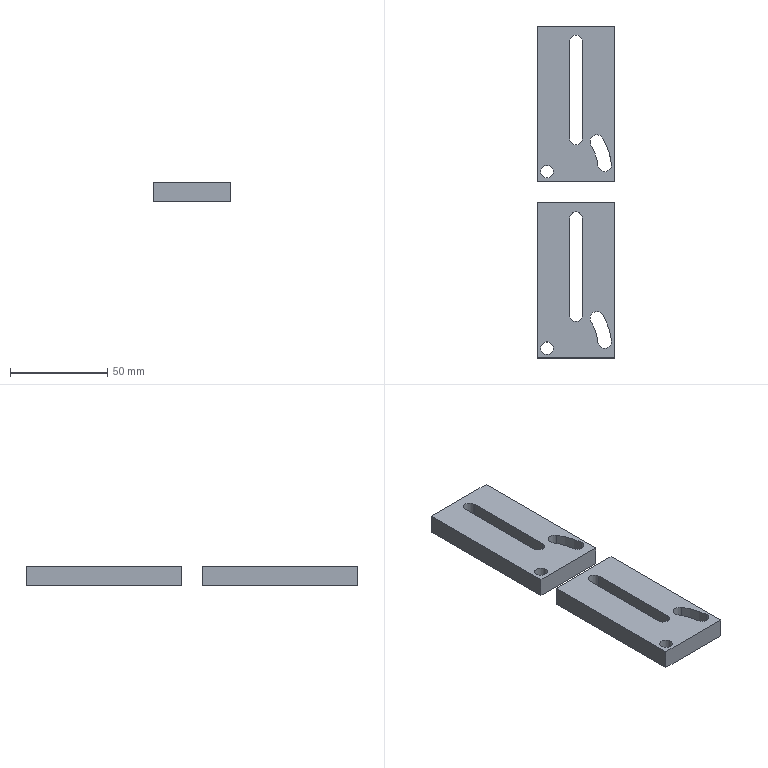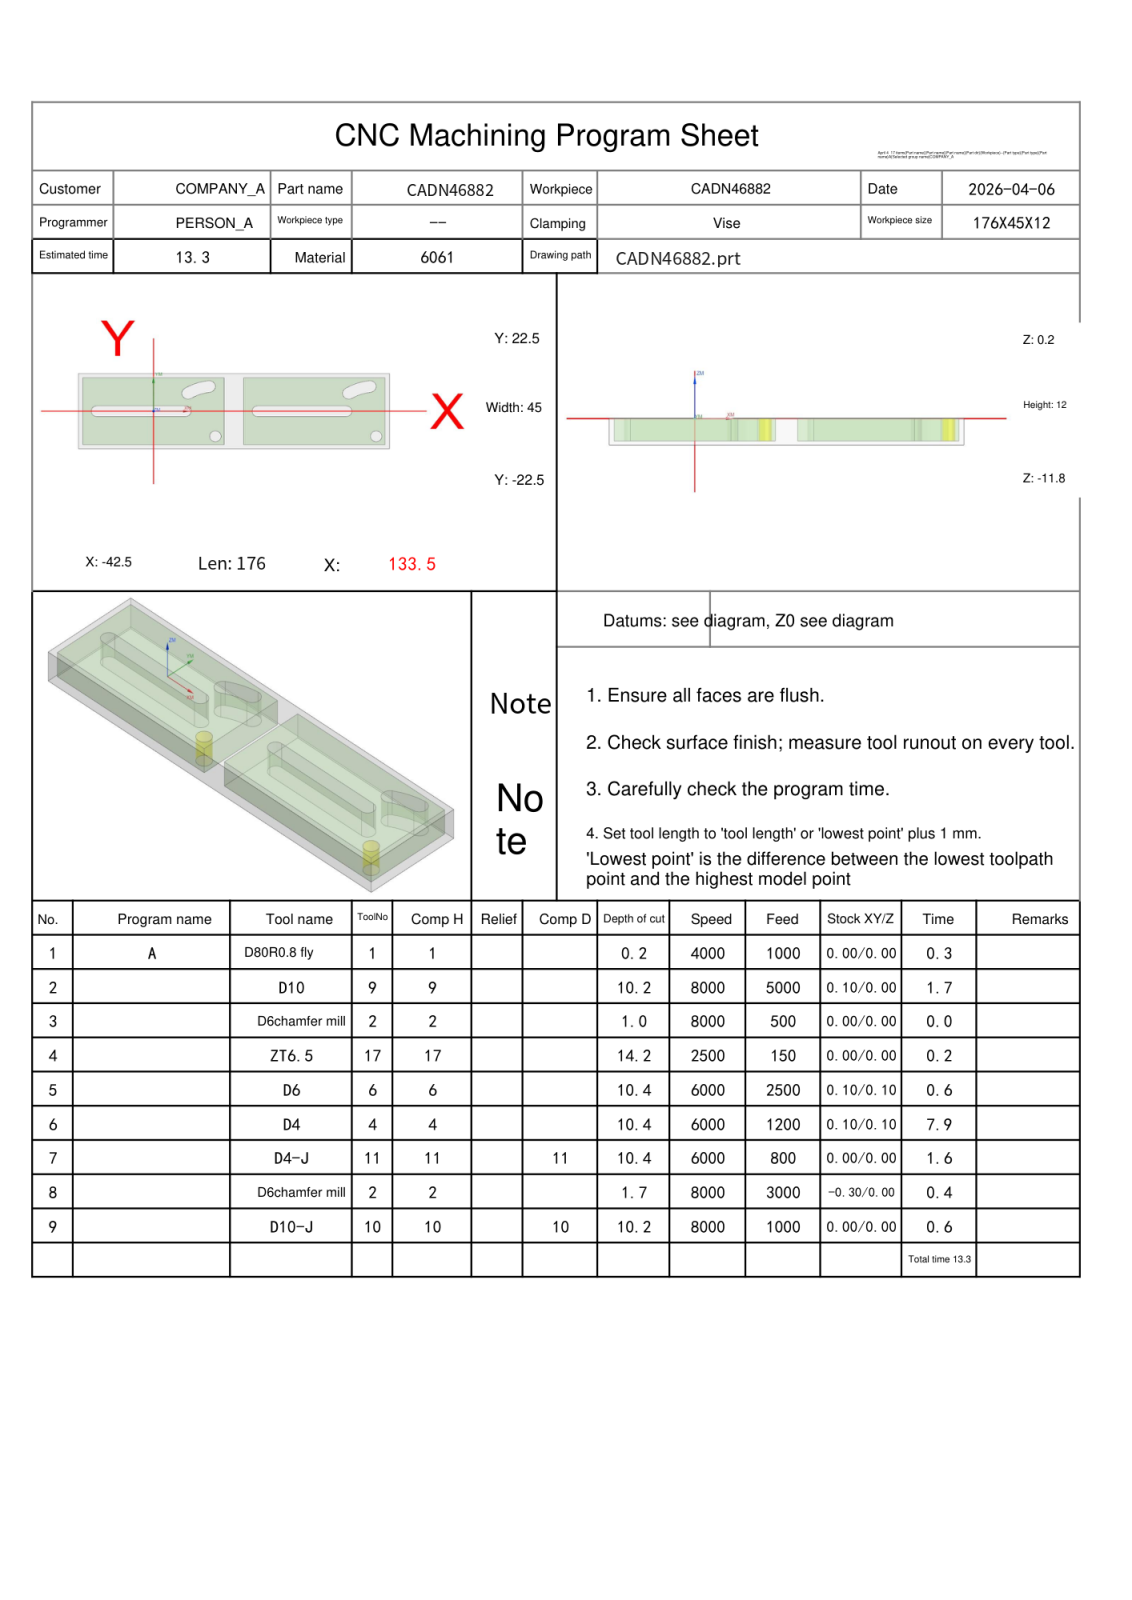NC program | NX | posted by the shop | part box 40 x 171 x 10 mm
Lines 1760 to 1806 of 1806:
N9 T10 M06
(D10-J  D=10. R=0. H=10 ce=0.00 di=0.00)
G00 G90 G54 X49.987 Y26.116 M03 S8000
G43 H10 Z20.
M08
Z-9.5
G01 Z-10. F1000.
G41 D10
X50.003 Y25.917
G03 X51. Y25. I.997 J.083
G01 X131.
G02 X136. Y20. I0.0 J-5.
G01 Y-20.
G02 X131. Y-25. I-5. J0.0
G01 X51.
G02 X46. Y-20. I0.0 J5.
G01 Y20.
G02 X51. Y25. I5. J0.0
G01 X51.5
G03 X52.5 Y26. I0.0 J1.
G01 G40 Y26.2
X45.149 Y23.453
G41 D10
X44.974 Y23.356
G03 X44.462 Y22.483 I.488 J-.873
X44.552 Y22.069 I1. J0.0
G02 X45. Y20. I-4.552 J-2.069
G01 Y-20.
G02 X40. Y-25. I-5. J0.0
G01 X-40.
G02 X-45. Y-20. I0.0 J5.
G01 Y20.
G02 X-40. Y25. I5. J0.0
G01 X40.
G02 X44.552 Y22.069 I0.0 J-5.
X44.736 Y21.604 I-4.552 J-2.069
G03 X45.683 Y20.925 I.947 J.321
X46.004 Y20.978 I0.0 J1.
G01 G40 X45.5 Y22.398
Z-9.5
G00 Z20.
M05
M09
G91 G28 Z0.0
G91 G28 Y0.0
M30
%